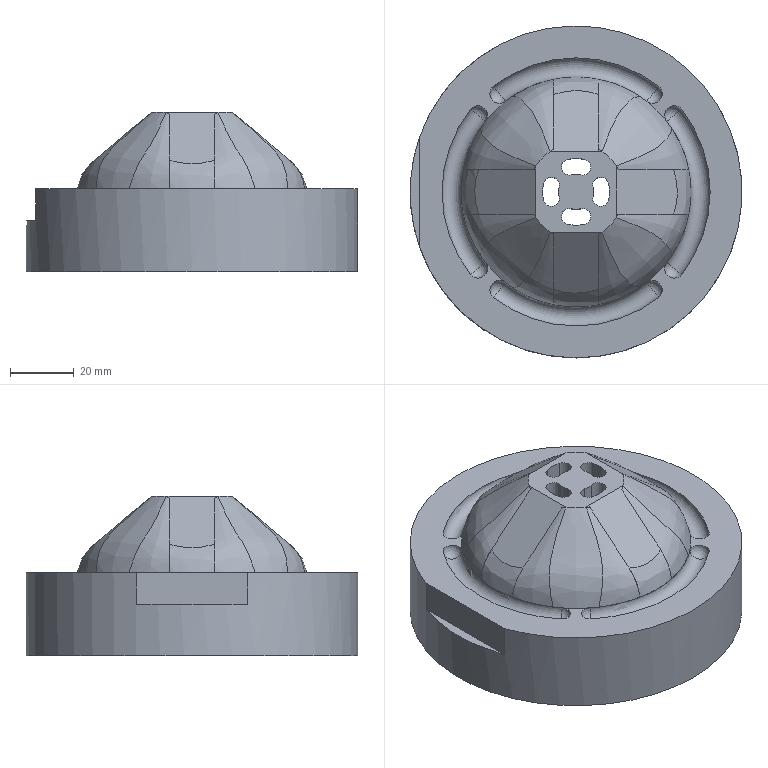NC program | NX | posted with a generic post | part box 104 x 104 x 49.86 mm
Lines 40750 to 41131 of 41131:
(ZLEVEL_PROFILE_COPY_COPY , TOOL : D10)
N81468 M6
N81470 G54
N81472 G17 G0 G90 X-57.86 Y-22.275 S3000 M3
N81474 G43 Z20. H0
N81476 Z-25.86
N81478 G94 G1 Z-28.86 F2000.
N81480 G3 X-54. Y-17.407 R5.
N81482 G1 Y17.407 F2500.
N81484 G3 X-57.86 Y22.275 R5.
N81486 G1 Z-25.86
N81488 G0 Z20.
N81490 Z-30.86
N81492 G1 Z-33.86 F2000.
N81494 G2 X-54. Y17.407 R5.
N81496 G1 Y-17.407 F2500.
N81498 G2 X-57.86 Y-22.275 R5.
N81500 G1 Z-30.86
N81502 G0 Z20.
N81504 M5
(PLUNGE_MILLING , TOOL : D20R0.8)
N81506 M6
N81508 G54
N81510 G17 G0 G90 X-58.973 Y-18.14 S1000 M3
N81512 G43 Z20. H0
N81514 Z-19.756
N81516 G94 G1 Z-22.756 F250.
N81518 Z-33.86
N81520 X-60.379 Y-19.729 Z-31.739
N81522 G0 Z-19.756
N81524 X-58.997 Y-17.637
N81526 G1 Z-22.756
N81528 Z-33.86
N81530 X-60.443 Y-19.189 Z-31.739
N81532 G0 Z-19.756
N81534 X-59. Y-17.133
N81536 G1 Z-22.756
N81538 Z-33.86
N81540 X-60.511 Y-18.622 Z-31.739
N81542 G0 Z-19.756
N81544 X-59. Y-16.629
N81546 G1 Z-22.756
N81548 Z-33.86
N81550 X-60.519 Y-18.11 Z-31.739
N81552 G0 Z-19.756
N81554 X-59. Y-16.125
N81556 G1 Z-22.756
N81558 Z-33.86
N81560 X-60.519 Y-17.606 Z-31.739
N81562 G0 Z-19.756
N81564 X-59. Y-15.621
N81566 G1 Z-22.756
N81568 Z-33.86
N81570 X-60.519 Y-17.102 Z-31.739
N81572 G0 Z-19.756
N81574 X-59. Y-15.117
N81576 G1 Z-22.756
N81578 Z-33.86
N81580 X-60.519 Y-16.598 Z-31.739
N81582 G0 Z-19.756
N81584 X-59. Y-14.613
N81586 G1 Z-22.756
N81588 Z-33.86
N81590 X-60.519 Y-16.095 Z-31.739
N81592 G0 Z-19.756
N81594 X-59. Y-14.11
N81596 G1 Z-22.756
N81598 Z-33.86
N81600 X-60.519 Y-15.591 Z-31.739
N81602 G0 Z-19.756
N81604 X-59. Y-13.606
N81606 G1 Z-22.756
N81608 Z-33.86
N81610 X-60.519 Y-15.087 Z-31.739
N81612 G0 Z-19.756
N81614 X-59. Y-13.102
N81616 G1 Z-22.756
N81618 Z-33.86
N81620 X-60.519 Y-14.583 Z-31.739
N81622 G0 Z-19.756
N81624 X-59. Y-12.598
N81626 G1 Z-22.756
N81628 Z-33.86
N81630 X-60.519 Y-14.079 Z-31.739
N81632 G0 Z-19.756
N81634 X-59. Y-12.094
N81636 G1 Z-22.756
N81638 Z-33.86
N81640 X-60.519 Y-13.575 Z-31.739
N81642 G0 Z-19.756
N81644 X-59. Y-11.59
N81646 G1 Z-22.756
N81648 Z-33.86
N81650 X-60.519 Y-13.071 Z-31.739
N81652 G0 Z-19.756
N81654 X-59. Y-11.086
N81656 G1 Z-22.756
N81658 Z-33.86
N81660 X-60.519 Y-12.567 Z-31.739
N81662 G0 Z-19.756
N81664 X-59. Y-10.582
N81666 G1 Z-22.756
N81668 Z-33.86
N81670 X-60.519 Y-12.063 Z-31.739
N81672 G0 Z-19.756
N81674 X-59. Y-10.078
N81676 G1 Z-22.756
N81678 Z-33.86
N81680 X-60.519 Y-11.559 Z-31.739
N81682 G0 Z-19.756
N81684 X-59. Y-9.574
N81686 G1 Z-22.756
N81688 Z-33.86
N81690 X-60.519 Y-11.055 Z-31.739
N81692 G0 Z-19.756
N81694 X-59. Y-9.07
N81696 G1 Z-22.756
N81698 Z-33.86
N81700 X-60.519 Y-10.552 Z-31.739
N81702 G0 Z-19.756
N81704 X-59. Y-8.567
N81706 G1 Z-22.756
N81708 Z-33.86
N81710 X-60.519 Y-10.048 Z-31.739
N81712 G0 Z-19.756
N81714 X-59. Y-8.063
N81716 G1 Z-22.756
N81718 Z-33.86
N81720 X-60.519 Y-9.544 Z-31.739
N81722 G0 Z-19.756
N81724 X-59. Y-7.559
N81726 G1 Z-22.756
N81728 Z-33.86
N81730 X-60.519 Y-9.04 Z-31.739
N81732 G0 Z-19.756
N81734 X-59. Y-7.055
N81736 G1 Z-22.756
N81738 Z-33.86
N81740 X-60.519 Y-8.536 Z-31.739
N81742 G0 Z-19.756
N81744 X-59. Y-6.551
N81746 G1 Z-22.756
N81748 Z-33.86
N81750 X-60.519 Y-8.032 Z-31.739
N81752 G0 Z-19.756
N81754 X-59. Y-6.047
N81756 G1 Z-22.756
N81758 Z-33.86
N81760 X-60.519 Y-7.528 Z-31.739
N81762 G0 Z-19.756
N81764 X-59. Y-5.543
N81766 G1 Z-22.756
N81768 Z-33.86
N81770 X-60.519 Y-7.024 Z-31.739
N81772 G0 Z-19.756
N81774 X-59. Y-5.039
N81776 G1 Z-22.756
N81778 Z-33.86
N81780 X-60.519 Y-6.52 Z-31.739
N81782 G0 Z-19.756
N81784 X-59. Y-4.535
N81786 G1 Z-22.756
N81788 Z-33.86
N81790 X-60.519 Y-6.016 Z-31.739
N81792 G0 Z-19.756
N81794 X-59. Y-4.031
N81796 G1 Z-22.756
N81798 Z-33.86
N81800 X-60.519 Y-5.512 Z-31.739
N81802 G0 Z-19.756
N81804 X-59. Y-3.527
N81806 G1 Z-22.756
N81808 Z-33.86
N81810 X-60.519 Y-5.009 Z-31.739
N81812 G0 Z-19.756
N81814 X-59. Y-3.023
N81816 G1 Z-22.756
N81818 Z-33.86
N81820 X-60.519 Y-4.505 Z-31.739
N81822 G0 Z-19.756
N81824 X-59. Y-2.52
N81826 G1 Z-22.756
N81828 Z-33.86
N81830 X-60.519 Y-4.001 Z-31.739
N81832 G0 Z-19.756
N81834 X-59. Y-2.016
N81836 G1 Z-22.756
N81838 Z-33.86
N81840 X-60.519 Y-3.497 Z-31.739
N81842 G0 Z-19.756
N81844 X-59. Y-1.512
N81846 G1 Z-22.756
N81848 Z-33.86
N81850 X-60.519 Y-2.993 Z-31.739
N81852 G0 Z-19.756
N81854 X-59. Y-1.008
N81856 G1 Z-22.756
N81858 Z-33.86
N81860 X-60.519 Y-2.489 Z-31.739
N81862 G0 Z-19.756
N81864 X-59. Y-0.504
N81866 G1 Z-22.756
N81868 Z-33.86
N81870 X-60.519 Y-1.985 Z-31.739
N81872 G0 Z-19.756
N81874 X-59. Y0.
N81876 G1 Z-22.756
N81878 Z-33.86
N81880 X-60.519 Y-1.481 Z-31.739
N81882 G0 Z-19.756
N81884 X-59. Y0.504
N81886 G1 Z-22.756
N81888 Z-33.86
N81890 X-60.519 Y-0.977 Z-31.739
N81892 G0 Z-19.756
N81894 X-59. Y1.008
N81896 G1 Z-22.756
N81898 Z-33.86
N81900 X-60.519 Y-0.473 Z-31.739
N81902 G0 Z-19.756
N81904 X-59. Y1.512
N81906 G1 Z-22.756
N81908 Z-33.86
N81910 X-60.519 Y0.031 Z-31.739
N81912 G0 Z-19.756
N81914 X-59. Y2.016
N81916 G1 Z-22.756
N81918 Z-33.86
N81920 X-60.519 Y0.535 Z-31.739
N81922 G0 Z-19.756
N81924 X-59. Y2.52
N81926 G1 Z-22.756
N81928 Z-33.86
N81930 X-60.519 Y1.038 Z-31.739
N81932 G0 Z-19.756
N81934 X-59. Y3.023
N81936 G1 Z-22.756
N81938 Z-33.86
N81940 X-60.519 Y1.542 Z-31.739
N81942 G0 Z-19.756
N81944 X-59. Y3.527
N81946 G1 Z-22.756
N81948 Z-33.86
N81950 X-60.519 Y2.046 Z-31.739
N81952 G0 Z-19.756
N81954 X-59. Y4.031
N81956 G1 Z-22.756
N81958 Z-33.86
N81960 X-60.519 Y2.55 Z-31.739
N81962 G0 Z-19.756
N81964 X-59. Y4.535
N81966 G1 Z-22.756
N81968 Z-33.86
N81970 X-60.519 Y3.054 Z-31.739
N81972 G0 Z-19.756
N81974 X-59. Y5.039
N81976 G1 Z-22.756
N81978 Z-33.86
N81980 X-60.519 Y3.558 Z-31.739
N81982 G0 Z-19.756
N81984 X-59. Y5.543
N81986 G1 Z-22.756
N81988 Z-33.86
N81990 X-60.519 Y4.062 Z-31.739
N81992 G0 Z-19.756
N81994 X-59. Y6.047
N81996 G1 Z-22.756
N81998 Z-33.86
N82000 X-60.519 Y4.566 Z-31.739
N82002 G0 Z-19.756
N82004 X-59. Y6.551
N82006 G1 Z-22.756
N82008 Z-33.86
N82010 X-60.519 Y5.07 Z-31.739
N82012 G0 Z-19.756
N82014 X-59. Y7.055
N82016 G1 Z-22.756
N82018 Z-33.86
N82020 X-60.519 Y5.574 Z-31.739
N82022 G0 Z-19.756
N82024 X-59. Y7.559
N82026 G1 Z-22.756
N82028 Z-33.86
N82030 X-60.519 Y6.078 Z-31.739
N82032 G0 Z-19.756
N82034 X-59. Y8.063
N82036 G1 Z-22.756
N82038 Z-33.86
N82040 X-60.519 Y6.581 Z-31.739
N82042 G0 Z-19.756
N82044 X-59. Y8.567
N82046 G1 Z-22.756
N82048 Z-33.86
N82050 X-60.519 Y7.085 Z-31.739
N82052 G0 Z-19.756
N82054 X-59. Y9.07
N82056 G1 Z-22.756
N82058 Z-33.86
N82060 X-60.519 Y7.589 Z-31.739
N82062 G0 Z-19.756
N82064 X-59. Y9.574
N82066 G1 Z-22.756
N82068 Z-33.86
N82070 X-60.519 Y8.093 Z-31.739
N82072 G0 Z-19.756
N82074 X-59. Y10.078
N82076 G1 Z-22.756
N82078 Z-33.86
N82080 X-60.519 Y8.597 Z-31.739
N82082 G0 Z-19.756
N82084 X-59. Y10.582
N82086 G1 Z-22.756
N82088 Z-33.86
N82090 X-60.519 Y9.101 Z-31.739
N82092 G0 Z-19.756
N82094 X-59. Y11.086
N82096 G1 Z-22.756
N82098 Z-33.86
N82100 X-60.519 Y9.605 Z-31.739
N82102 G0 Z-19.756
N82104 X-59. Y11.59
N82106 G1 Z-22.756
N82108 Z-33.86
N82110 X-60.519 Y10.109 Z-31.739
N82112 G0 Z-19.756
N82114 X-59. Y12.094
N82116 G1 Z-22.756
N82118 Z-33.86
N82120 X-60.519 Y10.613 Z-31.739
N82122 G0 Z-19.756
N82124 X-59. Y12.598
N82126 G1 Z-22.756
N82128 Z-33.86
N82130 X-60.519 Y11.117 Z-31.739
N82132 G0 Z-19.756
N82134 X-59. Y13.102
N82136 G1 Z-22.756
N82138 Z-33.86
N82140 X-60.519 Y11.621 Z-31.739
N82142 G0 Z-19.756
N82144 X-59. Y13.606
N82146 G1 Z-22.756
N82148 Z-33.86
N82150 X-60.519 Y12.124 Z-31.739
N82152 G0 Z-19.756
N82154 X-59. Y14.11
N82156 G1 Z-22.756
N82158 Z-33.86
N82160 X-60.519 Y12.628 Z-31.739
N82162 G0 Z-19.756
N82164 X-59. Y14.613
N82166 G1 Z-22.756
N82168 Z-33.86
N82170 X-60.519 Y13.132 Z-31.739
N82172 G0 Z-19.756
N82174 X-59. Y15.117
N82176 G1 Z-22.756
N82178 Z-33.86
N82180 X-60.519 Y13.636 Z-31.739
N82182 G0 Z-19.756
N82184 X-59. Y15.621
N82186 G1 Z-22.756
N82188 Z-33.86
N82190 X-60.519 Y14.14 Z-31.739
N82192 G0 Z-19.756
N82194 X-59. Y16.125
N82196 G1 Z-22.756
N82198 Z-33.86
N82200 X-60.519 Y14.644 Z-31.739
N82202 G0 Z-19.756
N82204 X-59. Y16.629
N82206 G1 Z-22.756
N82208 Z-33.86
N82210 X-60.519 Y15.148 Z-31.739
N82212 G0 Z-19.756
N82214 Z20.
N82216 M5
N82218 M2